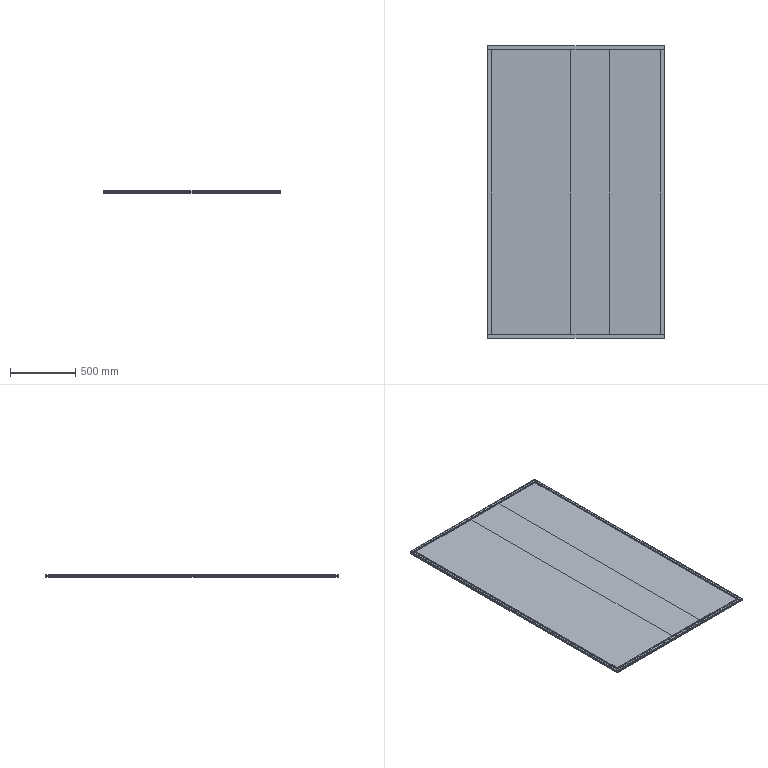Part | SolidWorks | features ICE 3, MirrorPattern 1, WeldMemberFeat 1, WeldmentFeature 1 | 5 solids | 175 faces | box 1350 x 2236 x 18 mm | volume 30026574 mm3 | plane 106 | cylinder 69 | commonest cylinder face diameters 1.1 x24 3.6 x20 5.8 x20 1 x5